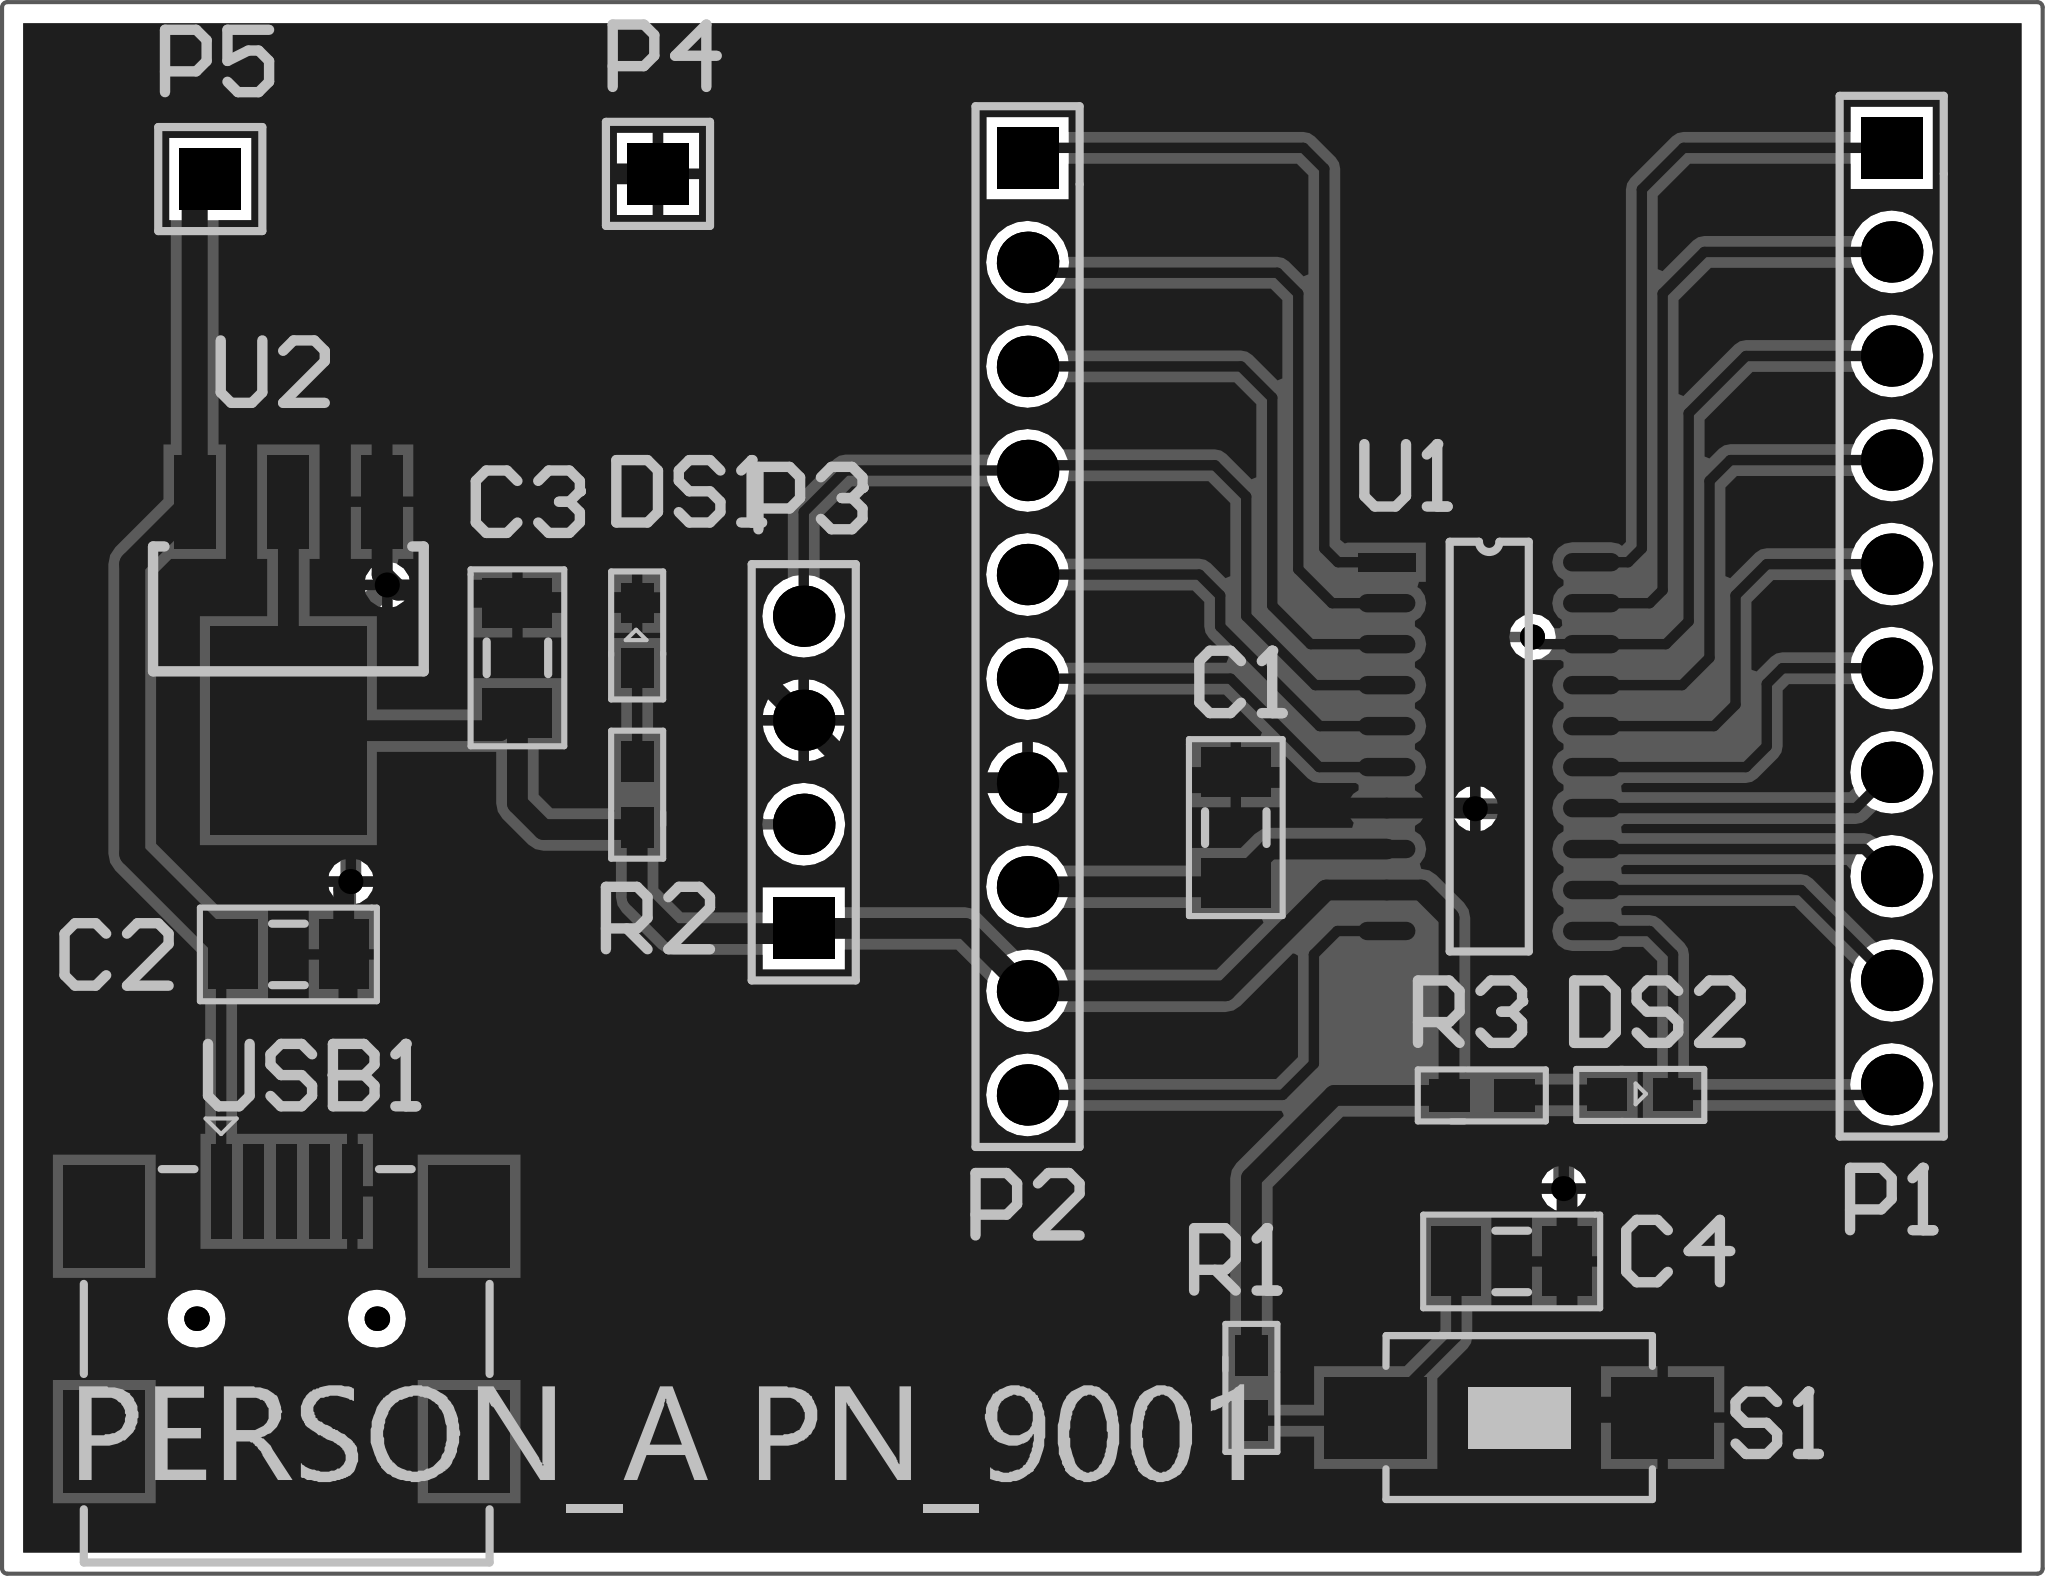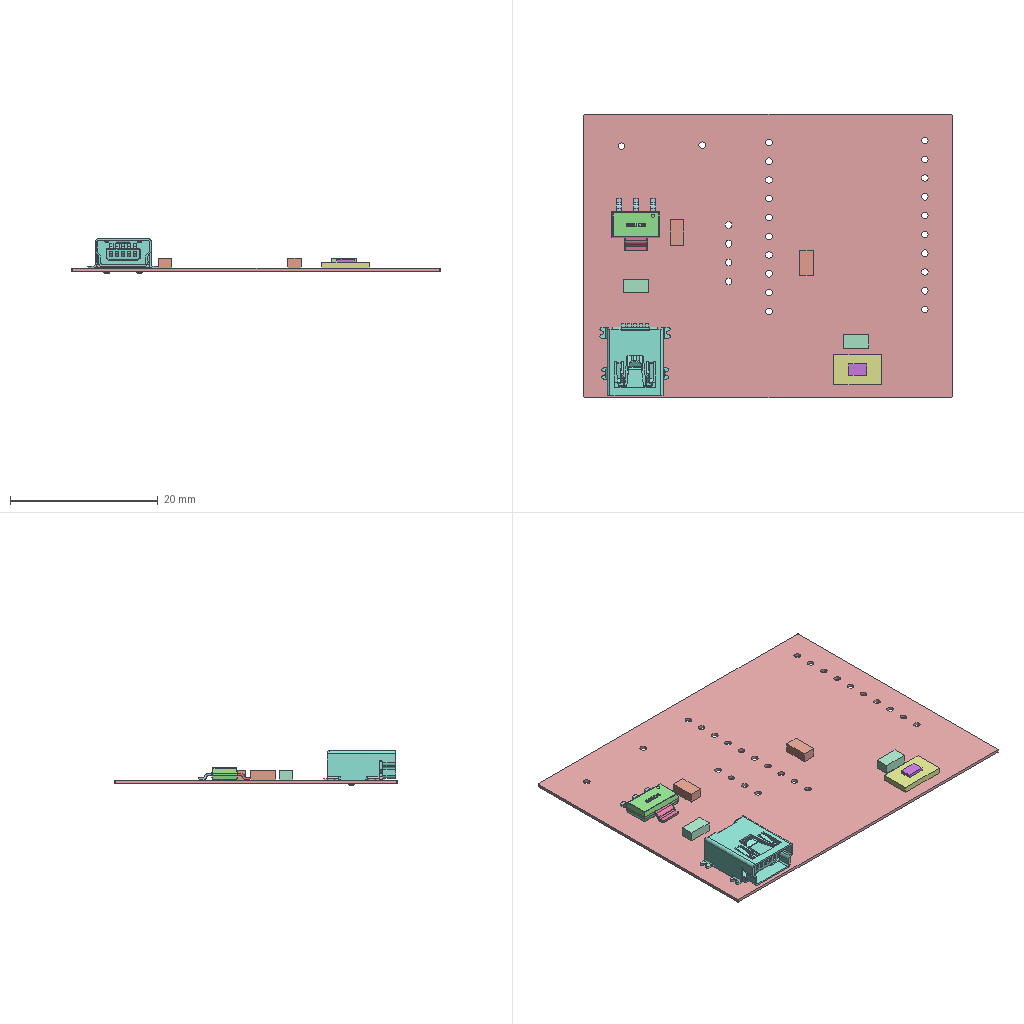Circuit board layout | Altium Designer | box 49.8 x 38.4 x 4.6 mm
Layer stack:
# Altium Designer layer stack of  (unit mm; dielectric type: 0 none, 1 core, 2 prepreg, 3 surface material)
index,name,kind,layer,copper_thickness_mm,dielectric_type,dielectric_thickness_mm,dielectric_material,dielectric_constant
0,Top Paste,other,,,,,,
1,Top Overlay,other,,,,,,
2,Top Solder,dielectric,,,3,0.0102,Solder Resist,3.5
3,Top Layer,copper,Top Layer,0.0356,,,,
4,Dielectric 1,dielectric,,,0,0.32,FR-4,4.8
5,Bottom Layer,copper,Bottom Layer,0.0356,,,,
6,Bottom Solder,dielectric,,,3,0.0102,Solder Resist,3.5
7,Bottom Overlay,other,,,,,,
8,Bottom Paste,other,,,,,,
# drill layer pairs: low layer,high layer
drill_pair,Top Layer,Bottom Layer
Part placement:
Designator,Comment,Layer,Footprint,Center-X(mm),Center-Y(mm),Rotation
USB1,MINI-USB,TopLayer,USB-MINI-A,109.052,98.225,0
U2,AMS1117,TopLayer,SOT223,109.093,115.316,180
U1,STM8S103F3,TopLayer,SOP-20,138.39,112.133,0
S1,SW-PB,TopLayer,SW_PB2_A1,139.121,95.758,270
R3,Res2,TopLayer,my0603,138.209,103.62,180
R2,Res2,TopLayer,my0603,117.602,110.96,270
R1,Res2,TopLayer,my0603,132.588,96.482,90
P5,HDR1X1,TopLayer,HDR1X1,107.188,125.984,0
P4,HDR1X1,TopLayer,HDR1X1,118.11,126.111,0
P3,Header 4,TopLayer,HDR1X4,121.666,111.506,90
P2,Header 10,TopLayer,HDR1X10,127.127,115.062,270
P1,Header 10,TopLayer,HDR1X10,148.209,115.316,270
DS2,LED2,TopLayer,my0603LED,142.075,103.632,360
DS1,LED2,TopLayer,my0603LED,117.602,114.846,90
C4,0.1UF,TopLayer,C1206,138.938,99.568,180
C3,0.1UF,TopLayer,C1206,114.681,114.3,270
C2,0.1UF,TopLayer,C1206,109.093,107.061,180
C1,0.1UF,TopLayer,C1206,132.207,110.156,270
Pad and via stacks:
# Altium Designer via and pad stacks of  (unit mm). Each distinct definition once, with the count of objects using it.
# via: kind,start_layer,end_layer,hole_mm,diameter_mm,mode(0 simple;1 top-mid-bottom;2 full stack),diameter_per_layer,count,example_net
# pad: kind,layer,hole_mm,hole_type(0 round;1 square;2 slot),plating,top_size,top_shape(1 round;2 rect;3 octagon;9 rounded rect),mid_size,bottom_size,mode,footprint,size_per_layer,count,example
pad,Top Layer,0,0,plated,1.4x0.45,1,1.4x0.45,1.4x0.45,0,SOP-20,,19,U1.11
pad,Top Layer,0,0,plated,1.4x0.45,2,1.4x0.45,1.4x0.45,0,SOP-20,,1,U1.1
pad,Top Layer,0,0,plated,1.7x1.2,2,1.7x1.2,1.7x1.2,0,C1206,,8,C1.1
pad,Top Layer,0,0,plated,1.016x2.286,2,1.016x2.286,1.016x2.286,0,SOT223,,3,U2.3
pad,Top Layer,0,0,plated,3.81x5.08,2,3.81x5.08,3.81x5.08,0,SOT223,,1,U2.2
pad,Top Layer,0,0,plated,2x2.5,2,2x2.5,2x2.5,0,USB-MINI-A,,4,USB1.0
pad,Top Layer,0,0,plated,0.5x2.3,2,0.5x2.3,0.5x2.3,0,USB-MINI-A,,5,USB1.1
pad,Top Layer,0,0,plated,1x0.8,2,1x0.8,1x0.8,0,my0603,,6,R1.1
pad,Top Layer,0,0,plated,2.5x2,2,2.5x2,2.5x2,0,SW_PB2_A1,,2,S1.1
pad,Top Layer,0,0,plated,0.965x0.8,2,0.965x0.8,0.965x0.8,0,my0603LED,,4,DS1.2
pad,Multi-Layer,0.9,0,plated,1.5x1.5,1,1.5x1.5,1.5x1.5,0,HDR1X10,,18,P1.3
pad,Multi-Layer,0.9,0,plated,1.5x1.5,2,1.5x1.5,1.5x1.5,0,HDR1X10,,2,P1.1
pad,Multi-Layer,0.9,0,unplated,0.6x0.6,1,0.6x0.6,0.6x0.6,0,USB-MINI-A,,2,USB1.MH1
pad,Multi-Layer,0.9,0,plated,1.5x1.5,1,1.5x1.5,1.5x1.5,0,HDR1X4,,3,P3.4
pad,Multi-Layer,0.9,0,plated,1.5x1.5,2,1.5x1.5,1.5x1.5,0,HDR1X4,,1,P3.1
pad,Multi-Layer,0.9,2,plated,1.5x1.5,2,1.5x1.5,1.5x1.5,0,HDR1X1,,2,P4.1
via,Top Layer,Bottom Layer,0.3048,0.6096,0,,5,GND
Copper pours:
name,layer,net,type(0 solid;1 hatched;2 none)
D,Bottom Layer,GND,0
D,Top Layer,GND,0
Design rules, without the lines most boards share:
# Altium Designer design rules of  (exported by Altium Designer, unit mm)
# columns: name | kind | enabled | priority | scope1 | scope2 | descriptor | typed fields (field=value)
SilkToSilkClearance | 55 | enabled | 1 | All | All | Silk to Silk (Clearance=0mil) (All),(All) |
SilkToSolderMaskClearance | 54 | enabled | 1 | IsPad | All | Silk To Solder Mask (Clearance=0mil) (IsPad),(All) |
MinimumSolderMaskSliver | 53 | enabled | 1 | All | All | Minimum Solder Mask Sliver (Gap=0mil) (All),(All) |
HoleToHoleClearance | 52 | enabled | 1 | All | All | Hole To Hole Clearance (Gap=10mil) (All),(All) | gap=0.254
DiffPairsRouting | 51 | enabled | 1 | All | All | Differential Pairs Uncoupled Length using the Gap Constraints (Min=10mil) (Max=10mil) (Prefered=10mil)  and Width Constraints (Min=15mil) (Max=15mil) (Prefered=15mil) (All) |
SolderMaskExpansion | 13 | enabled | 1 | All | All | Solder Mask Expansion (Expansion =4mil) (All) | expansion=0.1016
PasteMaskExpansion | 14 | enabled | 1 | All | All | Paste Mask Expansion (Expansion =0mil) (All) | expansion=0
RoutingVias | 11 | enabled | 1 | All | All | Routing Via (MinHoleWidth=28mil) (MaxHoleWidth=28mil) (PreferredHoleWidth=28mil) (MinWidth=50mil) (MaxWidth=50mil) (PreferedWidth=50mil) (All) | via_min_hole=0.7112 via_max_hole=0.7112 via_preferred_diameter=1.27 via_preferred_hole=0.7112
Width | 2 | enabled | 1 | All | All | Width Constraint (Min=10mil) (Max=39.37mil) (Preferred=10mil) (All) |
PolygonConnect | 20 | enabled | 1 | All | All | Polygon Connect Rule(Relief Connect )(Conductor Width=10mil) (Relief Angle=90 Angle) (Entries=4) (Air Gap Width=10mil) (All),(All) | connect_style(0=relief,1=direct,2=none)=0 relief_conductor_width=0.254 relief_entries=4
PlaneConnect | 6 | enabled | 1 | All | All | Power Plane Connect Rule(Relief Connect )(Expansion=20mil) (Conductor Width=10mil) (Air Gap=10mil) (Entries=4) (All) | relief_conductor_width=0.254 relief_entries=4 relief_expansion=0.508
Clearance | 0 | enabled | 1 | All | All | Clearance Constraint (Gap=10mil) (All),(All) | gap=0.254
Classes set for this board:
# Altium Designer classes of  (member kind: 0 net, 1 component, 2 from-to, 3 pad, 4 layer, 5 differential pair, 6 design channel, 7 polygon, 8 structure, 9 xSignal)
# columns: class name | member kind | superclass | members
Sheet1 | 1 | no | C1; C2; C3; C4; DS1; DS2; P1; P2; P3; P4; P5; R1; R2; R3; S1; U1; U2; USB1;